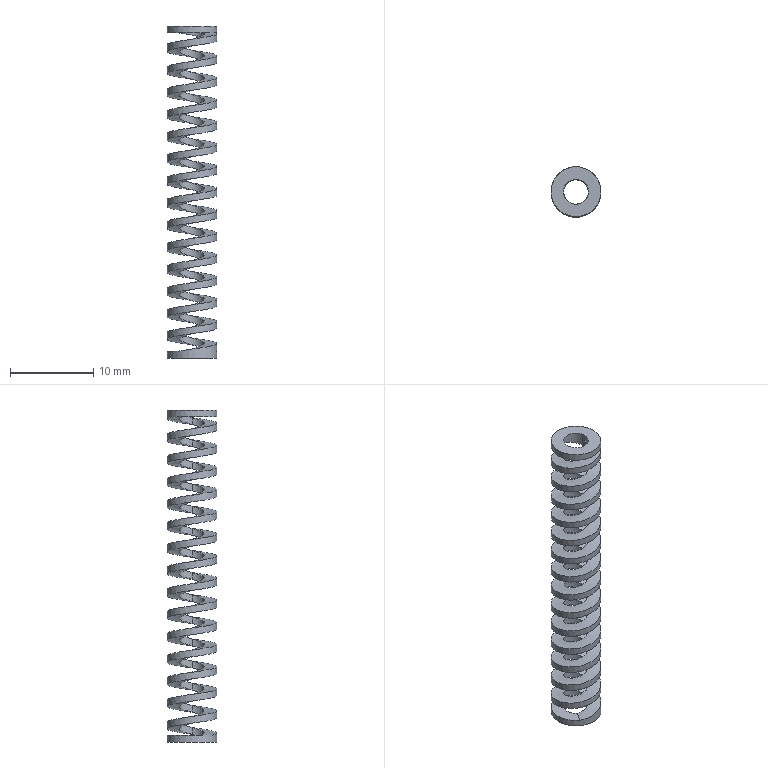Part | STEP file | 1 solid | 38 faces | box 6 x 6 x 40 mm | volume 281.648 mm3 | cylinder 32 | plane 4 | spline 2 | commonest cylinder face diameters 3 x16 6 x16